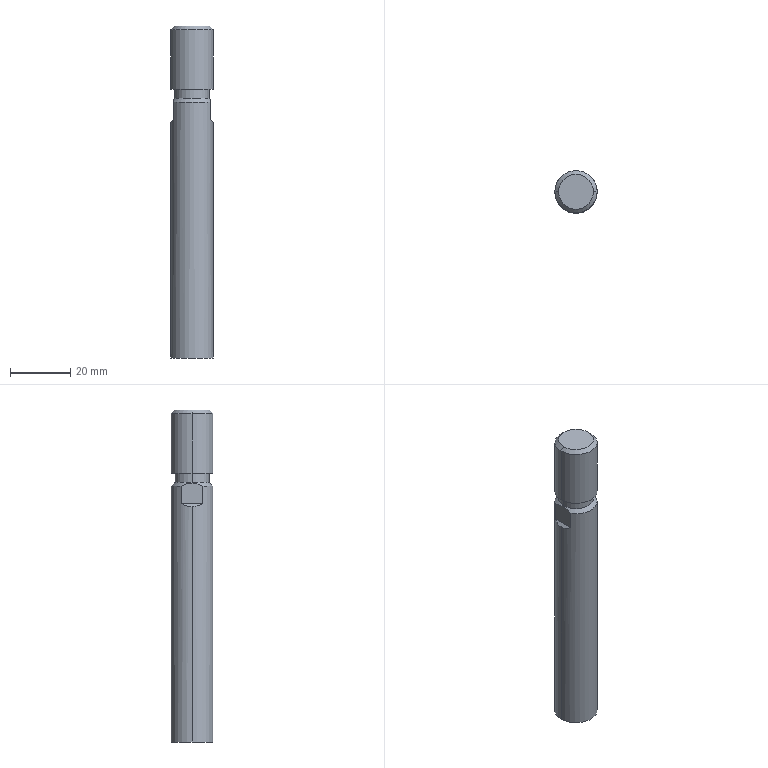Part | STEP file | rod_A_CDM2C40F_75_C76_0_ | 1 solid | 17 faces | box 14 x 14 x 110 mm | volume 16659 mm3 | plane 7 | cylinder 6 | cone 4 | commonest cylinder face diameters 14 x4 11.55 x2
STEP:
#1=CARTESIAN_POINT('',(7.,0.,-76.));
#2=VERTEX_POINT('',#1);
#3=CARTESIAN_POINT('',(-7.,0.,-76.));
#4=VERTEX_POINT('',#3);
#5=CARTESIAN_POINT('',(0.,0.,-76.));
#6=DIRECTION('',(0.,0.,1.));
#7=DIRECTION('',(1.,0.,0.));
#8=AXIS2_PLACEMENT_3D('',#5,#6,#7);
#9=CIRCLE('',#8,7.);
#10=EDGE_CURVE('',#2,#4,#9,.T.);
#11=ORIENTED_EDGE('',*,*,#10,.T.);
#12=CARTESIAN_POINT('',(-7.,0.,2.));
#13=VERTEX_POINT('',#12);
#14=CARTESIAN_POINT('',(-7.,0.,-76.));
#15=DIRECTION('',(0.,0.,1.));
#16=VECTOR('',#15,1000.);
#17=LINE('',#14,#16);
#18=EDGE_CURVE('',#4,#13,#17,.T.);
#19=ORIENTED_EDGE('',*,*,#18,.T.);
#20=CARTESIAN_POINT('',(-6.,3.606,3.));
#21=VERTEX_POINT('',#20);
#22=CARTESIAN_POINT('',(-7.,0.,2.));
#23=CARTESIAN_POINT('',(-7.,1.278,2.));
#24=CARTESIAN_POINT('',(-6.658,2.51,2.342));
#25=CARTESIAN_POINT('',(-6.,3.606,3.));
#26=(BOUNDED_CURVE()B_SPLINE_CURVE(3,(#22,#23,#24,#25),.UNSPECIFIED.,.F.,.F.)B_SPLINE_CURVE_WITH_KNOTS((4,4),(3.142,3.683),.UNSPECIFIED.)CURVE()GEOMETRIC_REPRESENTATION_ITEM()RATIONAL_B_SPLINE_CURVE((1.,0.9757,0.9757,1.))REPRESENTATION_ITEM(''));
#27=EDGE_CURVE('',#13,#21,#26,.T.);
#28=ORIENTED_EDGE('',*,*,#27,.T.);
#29=CARTESIAN_POINT('',(-6.,3.606,8.775));
#30=VERTEX_POINT('',#29);
#31=CARTESIAN_POINT('',(-6.,3.606,-76.));
#32=DIRECTION('',(0.,0.,1.));
#33=VECTOR('',#32,1000.);
#34=LINE('',#31,#33);
#35=EDGE_CURVE('',#21,#30,#34,.T.);
#36=ORIENTED_EDGE('',*,*,#35,.T.);
#37=CARTESIAN_POINT('',(6.,3.606,8.775));
#38=VERTEX_POINT('',#37);
#39=CARTESIAN_POINT('',(0.,0.,8.775));
#40=DIRECTION('',(0.,0.,1.));
#41=DIRECTION('',(1.,0.,0.));
#42=AXIS2_PLACEMENT_3D('',#39,#40,#41);
#43=CIRCLE('',#42,7.);
#44=EDGE_CURVE('',#38,#30,#43,.T.);
#45=ORIENTED_EDGE('',*,*,#44,.F.);
#46=CARTESIAN_POINT('',(6.,3.606,3.));
#47=VERTEX_POINT('',#46);
#48=CARTESIAN_POINT('',(6.,3.606,-76.));
#49=DIRECTION('',(0.,0.,-1.));
#50=VECTOR('',#49,1000.);
#51=LINE('',#48,#50);
#52=EDGE_CURVE('',#38,#47,#51,.T.);
#53=ORIENTED_EDGE('',*,*,#52,.T.);
#54=CARTESIAN_POINT('',(7.,0.,2.));
#55=VERTEX_POINT('',#54);
#56=CARTESIAN_POINT('',(6.,3.606,3.));
#57=CARTESIAN_POINT('',(6.658,2.51,2.342));
#58=CARTESIAN_POINT('',(7.,1.278,2.));
#59=CARTESIAN_POINT('',(7.,0.,2.));
#60=(BOUNDED_CURVE()B_SPLINE_CURVE(3,(#56,#57,#58,#59),.UNSPECIFIED.,.F.,.T.)B_SPLINE_CURVE_WITH_KNOTS((4,4),(2.6,3.142),.UNSPECIFIED.)CURVE()GEOMETRIC_REPRESENTATION_ITEM()RATIONAL_B_SPLINE_CURVE((1.,0.9757,0.9757,1.))REPRESENTATION_ITEM(''));
#61=EDGE_CURVE('',#47,#55,#60,.T.);
#62=ORIENTED_EDGE('',*,*,#61,.T.);
#63=CARTESIAN_POINT('',(7.,0.,-76.));
#64=DIRECTION('',(0.,0.,1.));
#65=VECTOR('',#64,1000.);
#66=LINE('',#63,#65);
#67=EDGE_CURVE('',#2,#55,#66,.T.);
#68=ORIENTED_EDGE('',*,*,#67,.F.);
#69=EDGE_LOOP('',(#11,#19,#28,#36,#45,#53,#62,#68));
#70=FACE_OUTER_BOUND('',#69,.T.);
#71=CARTESIAN_POINT('',(0.,0.,-76.));
#72=DIRECTION('',(0.,0.,1.));
#73=DIRECTION('',(1.,0.,0.));
#74=AXIS2_PLACEMENT_3D('',#71,#72,#73);
#75=CYLINDRICAL_SURFACE('',#74,7.);
#76=ADVANCED_FACE('',(#70),#75,.T.);
#77=CARTESIAN_POINT('',(5.775,0.,10.));
#78=VERTEX_POINT('',#77);
#79=CARTESIAN_POINT('',(-5.775,0.,10.));
#80=VERTEX_POINT('',#79);
#81=CARTESIAN_POINT('',(0.,0.,10.));
#82=DIRECTION('',(0.,0.,1.));
#83=DIRECTION('',(1.,0.,0.));
#84=AXIS2_PLACEMENT_3D('',#81,#82,#83);
#85=CIRCLE('',#84,5.775);
#86=EDGE_CURVE('',#78,#80,#85,.T.);
#87=ORIENTED_EDGE('',*,*,#86,.F.);
#88=CARTESIAN_POINT('',(6.,0.,9.775));
#89=VERTEX_POINT('',#88);
#90=CARTESIAN_POINT('',(7.,0.,8.775));
#91=DIRECTION('',(0.7071,0.,-0.7071));
#92=VECTOR('',#91,1000.);
#93=LINE('',#90,#92);
#94=EDGE_CURVE('',#78,#89,#93,.T.);
#95=ORIENTED_EDGE('',*,*,#94,.T.);
#96=CARTESIAN_POINT('',(6.,0.,9.775));
#97=CARTESIAN_POINT('',(6.,0.3144,9.775));
#98=CARTESIAN_POINT('',(6.,0.6332,9.75));
#99=CARTESIAN_POINT('',(6.,1.255,9.653));
#100=CARTESIAN_POINT('',(6.,1.561,9.582));
#101=CARTESIAN_POINT('',(6.,2.164,9.403));
#102=CARTESIAN_POINT('',(6.,2.462,9.295));
#103=CARTESIAN_POINT('',(6.,3.044,9.052));
#104=CARTESIAN_POINT('',(6.,3.328,8.918));
#105=CARTESIAN_POINT('',(6.,3.606,8.775));
#106=B_SPLINE_CURVE_WITH_KNOTS('',3,(#96,#97,#98,#99,#100,#101,#102,#103,#104,#105),.UNSPECIFIED.,.F.,.F.,(4,2,2,2,4),(0.01366,0.0146,0.01554,0.01648,0.01742),.UNSPECIFIED.);
#107=EDGE_CURVE('',#89,#38,#106,.T.);
#108=ORIENTED_EDGE('',*,*,#107,.T.);
#109=ORIENTED_EDGE('',*,*,#44,.T.);
#110=CARTESIAN_POINT('',(-6.,0.,9.775));
#111=VERTEX_POINT('',#110);
#112=CARTESIAN_POINT('',(-6.,3.606,8.775));
#113=CARTESIAN_POINT('',(-6.,3.328,8.918));
#114=CARTESIAN_POINT('',(-6.,3.044,9.052));
#115=CARTESIAN_POINT('',(-6.,2.462,9.295));
#116=CARTESIAN_POINT('',(-6.,2.164,9.403));
#117=CARTESIAN_POINT('',(-6.,1.561,9.582));
#118=CARTESIAN_POINT('',(-6.,1.255,9.653));
#119=CARTESIAN_POINT('',(-6.,0.6332,9.75));
#120=CARTESIAN_POINT('',(-6.,0.3144,9.775));
#121=CARTESIAN_POINT('',(-6.,0.,9.775));
#122=B_SPLINE_CURVE_WITH_KNOTS('',3,(#112,#113,#114,#115,#116,#117,#118,#119,#120,#121),.UNSPECIFIED.,.F.,.F.,(4,2,2,2,4),(0.004778,0.005712,0.006646,0.00758,0.008514),.UNSPECIFIED.);
#123=EDGE_CURVE('',#30,#111,#122,.T.);
#124=ORIENTED_EDGE('',*,*,#123,.T.);
#125=CARTESIAN_POINT('',(-7.,0.,8.775));
#126=DIRECTION('',(-0.7071,0.,-0.7071));
#127=VECTOR('',#126,1000.);
#128=LINE('',#125,#127);
#129=EDGE_CURVE('',#80,#111,#128,.T.);
#130=ORIENTED_EDGE('',*,*,#129,.F.);
#131=EDGE_LOOP('',(#87,#95,#108,#109,#124,#130));
#132=FACE_OUTER_BOUND('',#131,.T.);
#133=CARTESIAN_POINT('',(0.,0.,8.775));
#134=DIRECTION('',(0.,0.,-1.));
#135=DIRECTION('',(-1.,0.,0.));
#136=AXIS2_PLACEMENT_3D('',#133,#134,#135);
#137=CONICAL_SURFACE('',#136,7.,0.7854);
#138=ADVANCED_FACE('',(#132),#137,.T.);
#139=ORIENTED_EDGE('',*,*,#86,.T.);
#140=CARTESIAN_POINT('',(-5.775,0.,13.));
#141=VERTEX_POINT('',#140);
#142=CARTESIAN_POINT('',(-5.775,0.,-76.));
#143=DIRECTION('',(0.,0.,1.));
#144=VECTOR('',#143,1000.);
#145=LINE('',#142,#144);
#146=EDGE_CURVE('',#80,#141,#145,.T.);
#147=ORIENTED_EDGE('',*,*,#146,.T.);
#148=CARTESIAN_POINT('',(5.775,0.,13.));
#149=VERTEX_POINT('',#148);
#150=CARTESIAN_POINT('',(0.,0.,13.));
#151=DIRECTION('',(0.,0.,1.));
#152=DIRECTION('',(1.,0.,0.));
#153=AXIS2_PLACEMENT_3D('',#150,#151,#152);
#154=CIRCLE('',#153,5.775);
#155=EDGE_CURVE('',#149,#141,#154,.T.);
#156=ORIENTED_EDGE('',*,*,#155,.F.);
#157=CARTESIAN_POINT('',(5.775,0.,-76.));
#158=DIRECTION('',(0.,0.,1.));
#159=VECTOR('',#158,1000.);
#160=LINE('',#157,#159);
#161=EDGE_CURVE('',#78,#149,#160,.T.);
#162=ORIENTED_EDGE('',*,*,#161,.F.);
#163=EDGE_LOOP('',(#139,#147,#156,#162));
#164=FACE_OUTER_BOUND('',#163,.T.);
#165=CARTESIAN_POINT('',(0.,0.,-76.));
#166=DIRECTION('',(0.,0.,1.));
#167=DIRECTION('',(1.,0.,0.));
#168=AXIS2_PLACEMENT_3D('',#165,#166,#167);
#169=CYLINDRICAL_SURFACE('',#168,5.775);
#170=ADVANCED_FACE('',(#164),#169,.T.);
#171=CARTESIAN_POINT('',(7.,0.,13.));
#172=VERTEX_POINT('',#171);
#173=CARTESIAN_POINT('',(-7.,0.,13.));
#174=VERTEX_POINT('',#173);
#175=CARTESIAN_POINT('',(0.,0.,13.));
#176=DIRECTION('',(0.,0.,1.));
#177=DIRECTION('',(1.,0.,0.));
#178=AXIS2_PLACEMENT_3D('',#175,#176,#177);
#179=CIRCLE('',#178,7.);
#180=EDGE_CURVE('',#172,#174,#179,.T.);
#181=ORIENTED_EDGE('',*,*,#180,.T.);
#182=CARTESIAN_POINT('',(-7.,0.,32.775));
#183=VERTEX_POINT('',#182);
#184=CARTESIAN_POINT('',(-7.,0.,-76.));
#185=DIRECTION('',(0.,0.,1.));
#186=VECTOR('',#185,1000.);
#187=LINE('',#184,#186);
#188=EDGE_CURVE('',#174,#183,#187,.T.);
#189=ORIENTED_EDGE('',*,*,#188,.T.);
#190=CARTESIAN_POINT('',(7.,0.,32.775));
#191=VERTEX_POINT('',#190);
#192=CARTESIAN_POINT('',(0.,0.,32.775));
#193=DIRECTION('',(0.,0.,1.));
#194=DIRECTION('',(1.,0.,0.));
#195=AXIS2_PLACEMENT_3D('',#192,#193,#194);
#196=CIRCLE('',#195,7.);
#197=EDGE_CURVE('',#191,#183,#196,.T.);
#198=ORIENTED_EDGE('',*,*,#197,.F.);
#199=CARTESIAN_POINT('',(7.,0.,-76.));
#200=DIRECTION('',(0.,0.,1.));
#201=VECTOR('',#200,1000.);
#202=LINE('',#199,#201);
#203=EDGE_CURVE('',#172,#191,#202,.T.);
#204=ORIENTED_EDGE('',*,*,#203,.F.);
#205=EDGE_LOOP('',(#181,#189,#198,#204));
#206=FACE_OUTER_BOUND('',#205,.T.);
#207=CARTESIAN_POINT('',(0.,0.,-76.));
#208=DIRECTION('',(0.,0.,1.));
#209=DIRECTION('',(1.,0.,0.));
#210=AXIS2_PLACEMENT_3D('',#207,#208,#209);
#211=CYLINDRICAL_SURFACE('',#210,7.);
#212=ADVANCED_FACE('',(#206),#211,.T.);
#213=CARTESIAN_POINT('',(5.775,0.,34.));
#214=VERTEX_POINT('',#213);
#215=CARTESIAN_POINT('',(-5.775,0.,34.));
#216=VERTEX_POINT('',#215);
#217=CARTESIAN_POINT('',(0.,0.,34.));
#218=DIRECTION('',(0.,0.,1.));
#219=DIRECTION('',(1.,0.,0.));
#220=AXIS2_PLACEMENT_3D('',#217,#218,#219);
#221=CIRCLE('',#220,5.775);
#222=EDGE_CURVE('',#214,#216,#221,.T.);
#223=ORIENTED_EDGE('',*,*,#222,.F.);
#224=CARTESIAN_POINT('',(7.,0.,32.775));
#225=DIRECTION('',(0.7071,0.,-0.7071));
#226=VECTOR('',#225,1000.);
#227=LINE('',#224,#226);
#228=EDGE_CURVE('',#214,#191,#227,.T.);
#229=ORIENTED_EDGE('',*,*,#228,.T.);
#230=ORIENTED_EDGE('',*,*,#197,.T.);
#231=CARTESIAN_POINT('',(-7.,0.,32.775));
#232=DIRECTION('',(-0.7071,0.,-0.7071));
#233=VECTOR('',#232,1000.);
#234=LINE('',#231,#233);
#235=EDGE_CURVE('',#216,#183,#234,.T.);
#236=ORIENTED_EDGE('',*,*,#235,.F.);
#237=EDGE_LOOP('',(#223,#229,#230,#236));
#238=FACE_OUTER_BOUND('',#237,.T.);
#239=CARTESIAN_POINT('',(0.,0.,32.775));
#240=DIRECTION('',(0.,0.,-1.));
#241=DIRECTION('',(-1.,0.,0.));
#242=AXIS2_PLACEMENT_3D('',#239,#240,#241);
#243=CONICAL_SURFACE('',#242,7.,0.7854);
#244=ADVANCED_FACE('',(#238),#243,.T.);
#245=CARTESIAN_POINT('',(0.,0.,34.));
#246=DIRECTION('',(0.,0.,1.));
#247=DIRECTION('',(1.,0.,0.));
#248=AXIS2_PLACEMENT_3D('',#245,#246,#247);
#249=CIRCLE('',#248,5.775);
#250=EDGE_CURVE('',#216,#214,#249,.T.);
#251=ORIENTED_EDGE('',*,*,#250,.T.);
#252=ORIENTED_EDGE('',*,*,#222,.T.);
#253=EDGE_LOOP('',(#251,#252));
#254=FACE_OUTER_BOUND('',#253,.T.);
#255=CARTESIAN_POINT('',(0.,0.,34.));
#256=DIRECTION('',(0.,0.,-1.));
#257=DIRECTION('',(-1.,0.,0.));
#258=AXIS2_PLACEMENT_3D('',#255,#256,#257);
#259=PLANE('',#258);
#260=ADVANCED_FACE('',(#254),#259,.F.);
#261=ORIENTED_EDGE('',*,*,#228,.F.);
#262=ORIENTED_EDGE('',*,*,#250,.F.);
#263=ORIENTED_EDGE('',*,*,#235,.T.);
#264=CARTESIAN_POINT('',(0.,0.,32.775));
#265=DIRECTION('',(0.,0.,1.));
#266=DIRECTION('',(1.,0.,0.));
#267=AXIS2_PLACEMENT_3D('',#264,#265,#266);
#268=CIRCLE('',#267,7.);
#269=EDGE_CURVE('',#183,#191,#268,.T.);
#270=ORIENTED_EDGE('',*,*,#269,.T.);
#271=EDGE_LOOP('',(#261,#262,#263,#270));
#272=FACE_OUTER_BOUND('',#271,.T.);
#273=CARTESIAN_POINT('',(0.,0.,32.775));
#274=DIRECTION('',(0.,0.,-1.));
#275=DIRECTION('',(-1.,0.,0.));
#276=AXIS2_PLACEMENT_3D('',#273,#274,#275);
#277=CONICAL_SURFACE('',#276,7.,0.7854);
#278=ADVANCED_FACE('',(#272),#277,.T.);
#279=ORIENTED_EDGE('',*,*,#188,.F.);
#280=CARTESIAN_POINT('',(0.,0.,13.));
#281=DIRECTION('',(0.,0.,1.));
#282=DIRECTION('',(1.,0.,0.));
#283=AXIS2_PLACEMENT_3D('',#280,#281,#282);
#284=CIRCLE('',#283,7.);
#285=EDGE_CURVE('',#174,#172,#284,.T.);
#286=ORIENTED_EDGE('',*,*,#285,.T.);
#287=ORIENTED_EDGE('',*,*,#203,.T.);
#288=ORIENTED_EDGE('',*,*,#269,.F.);
#289=EDGE_LOOP('',(#279,#286,#287,#288));
#290=FACE_OUTER_BOUND('',#289,.T.);
#291=CARTESIAN_POINT('',(0.,0.,-76.));
#292=DIRECTION('',(0.,0.,1.));
#293=DIRECTION('',(1.,0.,0.));
#294=AXIS2_PLACEMENT_3D('',#291,#292,#293);
#295=CYLINDRICAL_SURFACE('',#294,7.);
#296=ADVANCED_FACE('',(#290),#295,.T.);
#297=ORIENTED_EDGE('',*,*,#180,.F.);
#298=ORIENTED_EDGE('',*,*,#285,.F.);
#299=EDGE_LOOP('',(#297,#298));
#300=FACE_OUTER_BOUND('',#299,.T.);
#301=ORIENTED_EDGE('',*,*,#155,.T.);
#302=CARTESIAN_POINT('',(0.,0.,13.));
#303=DIRECTION('',(0.,0.,1.));
#304=DIRECTION('',(1.,0.,0.));
#305=AXIS2_PLACEMENT_3D('',#302,#303,#304);
#306=CIRCLE('',#305,5.775);
#307=EDGE_CURVE('',#141,#149,#306,.T.);
#308=ORIENTED_EDGE('',*,*,#307,.T.);
#309=EDGE_LOOP('',(#301,#308));
#310=FACE_BOUND('',#309,.T.);
#311=CARTESIAN_POINT('',(0.,7.,13.));
#312=DIRECTION('',(0.,0.,1.));
#313=DIRECTION('',(1.,0.,0.));
#314=AXIS2_PLACEMENT_3D('',#311,#312,#313);
#315=PLANE('',#314);
#316=ADVANCED_FACE('',(#300,#310),#315,.F.);
#317=ORIENTED_EDGE('',*,*,#146,.F.);
#318=CARTESIAN_POINT('',(0.,0.,10.));
#319=DIRECTION('',(0.,0.,1.));
#320=DIRECTION('',(1.,0.,0.));
#321=AXIS2_PLACEMENT_3D('',#318,#319,#320);
#322=CIRCLE('',#321,5.775);
#323=EDGE_CURVE('',#80,#78,#322,.T.);
#324=ORIENTED_EDGE('',*,*,#323,.T.);
#325=ORIENTED_EDGE('',*,*,#161,.T.);
#326=ORIENTED_EDGE('',*,*,#307,.F.);
#327=EDGE_LOOP('',(#317,#324,#325,#326));
#328=FACE_OUTER_BOUND('',#327,.T.);
#329=CARTESIAN_POINT('',(0.,0.,-76.));
#330=DIRECTION('',(0.,0.,1.));
#331=DIRECTION('',(1.,0.,0.));
#332=AXIS2_PLACEMENT_3D('',#329,#330,#331);
#333=CYLINDRICAL_SURFACE('',#332,5.775);
#334=ADVANCED_FACE('',(#328),#333,.T.);
#335=ORIENTED_EDGE('',*,*,#94,.F.);
#336=ORIENTED_EDGE('',*,*,#323,.F.);
#337=ORIENTED_EDGE('',*,*,#129,.T.);
#338=CARTESIAN_POINT('',(-6.,-3.606,8.775));
#339=VERTEX_POINT('',#338);
#340=CARTESIAN_POINT('',(-6.,0.,9.775));
#341=CARTESIAN_POINT('',(-6.,-0.3152,9.775));
#342=CARTESIAN_POINT('',(-6.,-0.628,9.75));
#343=CARTESIAN_POINT('',(-6.,-1.249,9.654));
#344=CARTESIAN_POINT('',(-6.,-1.559,9.582));
#345=CARTESIAN_POINT('',(-6.,-2.47,9.312));
#346=CARTESIAN_POINT('',(-6.,-3.047,9.063));
#347=CARTESIAN_POINT('',(-6.,-3.606,8.775));
#348=B_SPLINE_CURVE_WITH_KNOTS('',3,(#340,#341,#342,#343,#344,#345,#346,#347),.UNSPECIFIED.,.F.,.F.,(4,2,2,4),(0.008514,0.009451,0.01039,0.01226),.UNSPECIFIED.);
#349=EDGE_CURVE('',#111,#339,#348,.T.);
#350=ORIENTED_EDGE('',*,*,#349,.T.);
#351=CARTESIAN_POINT('',(6.,-3.606,8.775));
#352=VERTEX_POINT('',#351);
#353=CARTESIAN_POINT('',(0.,0.,8.775));
#354=DIRECTION('',(0.,0.,1.));
#355=DIRECTION('',(1.,0.,0.));
#356=AXIS2_PLACEMENT_3D('',#353,#354,#355);
#357=CIRCLE('',#356,7.);
#358=EDGE_CURVE('',#339,#352,#357,.T.);
#359=ORIENTED_EDGE('',*,*,#358,.T.);
#360=CARTESIAN_POINT('',(6.,-3.606,8.775));
#361=CARTESIAN_POINT('',(6.,-3.047,9.063));
#362=CARTESIAN_POINT('',(6.,-2.47,9.312));
#363=CARTESIAN_POINT('',(6.,-1.559,9.582));
#364=CARTESIAN_POINT('',(6.,-1.249,9.654));
#365=CARTESIAN_POINT('',(6.,-0.628,9.75));
#366=CARTESIAN_POINT('',(6.,-0.3152,9.775));
#367=CARTESIAN_POINT('',(6.,0.,9.775));
#368=B_SPLINE_CURVE_WITH_KNOTS('',3,(#360,#361,#362,#363,#364,#365,#366,#367),.UNSPECIFIED.,.F.,.F.,(4,2,2,4),(0.009896,0.01178,0.01272,0.01366),.UNSPECIFIED.);
#369=EDGE_CURVE('',#352,#89,#368,.T.);
#370=ORIENTED_EDGE('',*,*,#369,.T.);
#371=EDGE_LOOP('',(#335,#336,#337,#350,#359,#370));
#372=FACE_OUTER_BOUND('',#371,.T.);
#373=CARTESIAN_POINT('',(0.,0.,8.775));
#374=DIRECTION('',(0.,0.,-1.));
#375=DIRECTION('',(-1.,0.,0.));
#376=AXIS2_PLACEMENT_3D('',#373,#374,#375);
#377=CONICAL_SURFACE('',#376,7.,0.7854);
#378=ADVANCED_FACE('',(#372),#377,.T.);
#379=ORIENTED_EDGE('',*,*,#18,.F.);
#380=CARTESIAN_POINT('',(0.,0.,-76.));
#381=DIRECTION('',(0.,0.,1.));
#382=DIRECTION('',(1.,0.,0.));
#383=AXIS2_PLACEMENT_3D('',#380,#381,#382);
#384=CIRCLE('',#383,7.);
#385=EDGE_CURVE('',#4,#2,#384,.T.);
#386=ORIENTED_EDGE('',*,*,#385,.T.);
#387=ORIENTED_EDGE('',*,*,#67,.T.);
#388=CARTESIAN_POINT('',(6.,-3.606,3.));
#389=VERTEX_POINT('',#388);
#390=CARTESIAN_POINT('',(7.,0.,2.));
#391=CARTESIAN_POINT('',(7.,-1.278,2.));
#392=CARTESIAN_POINT('',(6.658,-2.51,2.342));
#393=CARTESIAN_POINT('',(6.,-3.606,3.));
#394=(BOUNDED_CURVE()B_SPLINE_CURVE(3,(#390,#391,#392,#393),.UNSPECIFIED.,.F.,.T.)B_SPLINE_CURVE_WITH_KNOTS((4,4),(3.142,3.683),.UNSPECIFIED.)CURVE()GEOMETRIC_REPRESENTATION_ITEM()RATIONAL_B_SPLINE_CURVE((1.,0.9757,0.9757,1.))REPRESENTATION_ITEM(''));
#395=EDGE_CURVE('',#55,#389,#394,.T.);
#396=ORIENTED_EDGE('',*,*,#395,.T.);
#397=CARTESIAN_POINT('',(6.,-3.606,-76.));
#398=DIRECTION('',(0.,0.,1.));
#399=VECTOR('',#398,1000.);
#400=LINE('',#397,#399);
#401=EDGE_CURVE('',#389,#352,#400,.T.);
#402=ORIENTED_EDGE('',*,*,#401,.T.);
#403=ORIENTED_EDGE('',*,*,#358,.F.);
#404=CARTESIAN_POINT('',(-6.,-3.606,3.));
#405=VERTEX_POINT('',#404);
#406=CARTESIAN_POINT('',(-6.,-3.606,-76.));
#407=DIRECTION('',(0.,0.,-1.));
#408=VECTOR('',#407,1000.);
#409=LINE('',#406,#408);
#410=EDGE_CURVE('',#339,#405,#409,.T.);
#411=ORIENTED_EDGE('',*,*,#410,.T.);
#412=CARTESIAN_POINT('',(-6.,-3.606,3.));
#413=CARTESIAN_POINT('',(-6.658,-2.51,2.342));
#414=CARTESIAN_POINT('',(-7.,-1.278,2.));
#415=CARTESIAN_POINT('',(-7.,0.,2.));
#416=(BOUNDED_CURVE()B_SPLINE_CURVE(3,(#412,#413,#414,#415),.UNSPECIFIED.,.F.,.F.)B_SPLINE_CURVE_WITH_KNOTS((4,4),(2.6,3.142),.UNSPECIFIED.)CURVE()GEOMETRIC_REPRESENTATION_ITEM()RATIONAL_B_SPLINE_CURVE((1.,0.9757,0.9757,1.))REPRESENTATION_ITEM(''));
#417=EDGE_CURVE('',#405,#13,#416,.T.);
#418=ORIENTED_EDGE('',*,*,#417,.T.);
#419=EDGE_LOOP('',(#379,#386,#387,#396,#402,#403,#411,#418));
#420=FACE_OUTER_BOUND('',#419,.T.);
#421=CARTESIAN_POINT('',(0.,0.,-76.));
#422=DIRECTION('',(0.,0.,1.));
#423=DIRECTION('',(1.,0.,0.));
#424=AXIS2_PLACEMENT_3D('',#421,#422,#423);
#425=CYLINDRICAL_SURFACE('',#424,7.);
#426=ADVANCED_FACE('',(#420),#425,.T.);
#427=ORIENTED_EDGE('',*,*,#10,.F.);
#428=ORIENTED_EDGE('',*,*,#385,.F.);
#429=EDGE_LOOP('',(#427,#428));
#430=FACE_OUTER_BOUND('',#429,.T.);
#431=CARTESIAN_POINT('',(0.,7.,-76.));
#432=DIRECTION('',(0.,0.,1.));
#433=DIRECTION('',(1.,0.,0.));
#434=AXIS2_PLACEMENT_3D('',#431,#432,#433);
#435=PLANE('',#434);
#436=ADVANCED_FACE('',(#430),#435,.F.);
#437=CARTESIAN_POINT('',(6.,-14.,3.));
#438=DIRECTION('',(0.,1.,0.));
#439=VECTOR('',#438,1000.);
#440=LINE('',#437,#439);
#441=EDGE_CURVE('',#389,#47,#440,.T.);
#442=ORIENTED_EDGE('',*,*,#441,.T.);
#443=ORIENTED_EDGE('',*,*,#52,.F.);
#444=ORIENTED_EDGE('',*,*,#107,.F.);
#445=ORIENTED_EDGE('',*,*,#369,.F.);
#446=ORIENTED_EDGE('',*,*,#401,.F.);
#447=EDGE_LOOP('',(#442,#443,#444,#445,#446));
#448=FACE_OUTER_BOUND('',#447,.T.);
#449=CARTESIAN_POINT('',(6.,-14.,3.));
#450=DIRECTION('',(-1.,0.,0.));
#451=DIRECTION('',(0.,0.,1.));
#452=AXIS2_PLACEMENT_3D('',#449,#450,#451);
#453=PLANE('',#452);
#454=ADVANCED_FACE('',(#448),#453,.F.);
#455=ORIENTED_EDGE('',*,*,#441,.F.);
#456=ORIENTED_EDGE('',*,*,#395,.F.);
#457=ORIENTED_EDGE('',*,*,#61,.F.);
#458=EDGE_LOOP('',(#455,#456,#457));
#459=FACE_OUTER_BOUND('',#458,.T.);
#460=CARTESIAN_POINT('',(7.,-14.,2.));
#461=DIRECTION('',(-0.7071,0.,-0.7071));
#462=DIRECTION('',(-0.7071,0.,0.7071));
#463=AXIS2_PLACEMENT_3D('',#460,#461,#462);
#464=PLANE('',#463);
#465=ADVANCED_FACE('',(#459),#464,.F.);
#466=CARTESIAN_POINT('',(-6.,-14.,3.));
#467=DIRECTION('',(0.,1.,0.));
#468=VECTOR('',#467,1000.);
#469=LINE('',#466,#468);
#470=EDGE_CURVE('',#405,#21,#469,.T.);
#471=ORIENTED_EDGE('',*,*,#470,.T.);
#472=ORIENTED_EDGE('',*,*,#27,.F.);
#473=ORIENTED_EDGE('',*,*,#417,.F.);
#474=EDGE_LOOP('',(#471,#472,#473));
#475=FACE_OUTER_BOUND('',#474,.T.);
#476=CARTESIAN_POINT('',(-6.,-14.,3.));
#477=DIRECTION('',(0.7071,0.,-0.7071));
#478=DIRECTION('',(-0.7071,0.,-0.7071));
#479=AXIS2_PLACEMENT_3D('',#476,#477,#478);
#480=PLANE('',#479);
#481=ADVANCED_FACE('',(#475),#480,.F.);
#482=ORIENTED_EDGE('',*,*,#470,.F.);
#483=ORIENTED_EDGE('',*,*,#410,.F.);
#484=ORIENTED_EDGE('',*,*,#349,.F.);
#485=ORIENTED_EDGE('',*,*,#123,.F.);
#486=ORIENTED_EDGE('',*,*,#35,.F.);
#487=EDGE_LOOP('',(#482,#483,#484,#485,#486));
#488=FACE_OUTER_BOUND('',#487,.T.);
#489=CARTESIAN_POINT('',(-6.,-14.,10.));
#490=DIRECTION('',(1.,0.,0.));
#491=DIRECTION('',(0.,0.,-1.));
#492=AXIS2_PLACEMENT_3D('',#489,#490,#491);
#493=PLANE('',#492);
#494=ADVANCED_FACE('',(#488),#493,.F.);
#495=CLOSED_SHELL('',(#76,#138,#170,#212,#244,#260,#278,#296,#316,#334,#378,#426,#436,#454,#465,#481,#494));
#496=MANIFOLD_SOLID_BREP('',#495);
#497=CARTESIAN_POINT('',(0.,0.,0.));
#498=DIRECTION('',(0.,0.,1.));
#499=DIRECTION('',(1.,0.,0.));
#500=AXIS2_PLACEMENT_3D('',#497,#498,#499);
#501=(LENGTH_UNIT()NAMED_UNIT(*)SI_UNIT(.MILLI.,.METRE.));
#502=UNCERTAINTY_MEASURE_WITH_UNIT(LENGTH_MEASURE(0.00001),#501,'','');
#503=(NAMED_UNIT(*)PLANE_ANGLE_UNIT()SI_UNIT($,.RADIAN.));
#504=(NAMED_UNIT(*)SI_UNIT($,.STERADIAN.)SOLID_ANGLE_UNIT());
#505=(GEOMETRIC_REPRESENTATION_CONTEXT(3)GLOBAL_UNCERTAINTY_ASSIGNED_CONTEXT((#502))GLOBAL_UNIT_ASSIGNED_CONTEXT((#501,#503,#504))REPRESENTATION_CONTEXT('',''));
#506=ADVANCED_BREP_SHAPE_REPRESENTATION('',(#496,#500),#505);